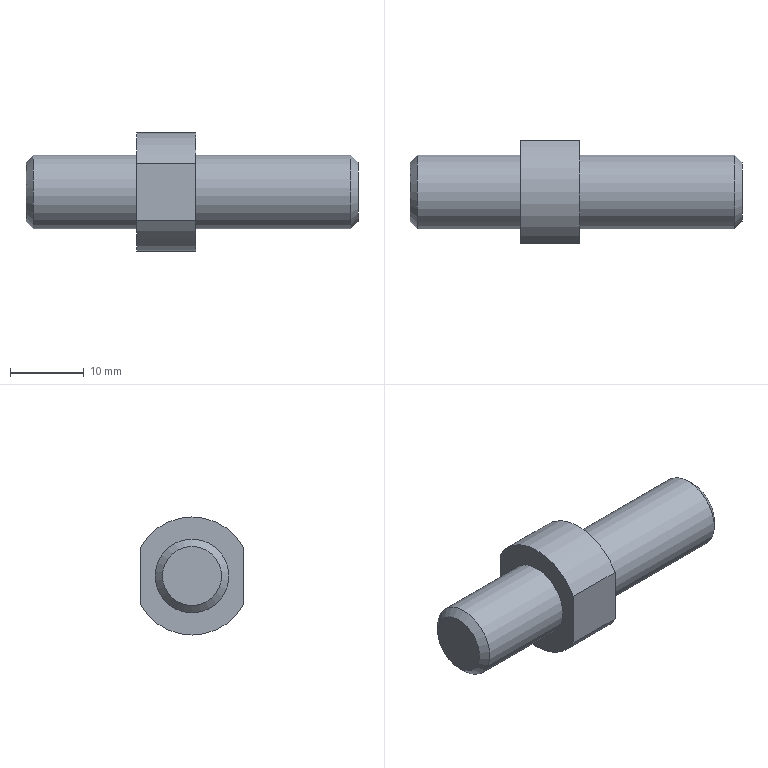Part | NX | 1 solid | 14 faces | box 45 x 14 x 16 mm | volume 4202 mm3 | plane 6 | cylinder 5 | cone 3 | commonest cylinder face diameters 10 x2 16 x2 4.2 x1
STEP:
#1=CARTESIAN_POINT('',(-19.,0.,5.));
#2=VERTEX_POINT('',#1);
#3=CARTESIAN_POINT('',(-19.,0.,0.));
#4=DIRECTION('',(-1.,0.,0.));
#5=DIRECTION('',(0.,0.,1.));
#6=AXIS2_PLACEMENT_3D('',#3,#4,#5);
#7=CIRCLE('',#6,5.);
#8=EDGE_CURVE('',#2,#2,#7,.T.);
#9=ORIENTED_EDGE('',*,*,#8,.F.);
#10=EDGE_LOOP('',(#9));
#11=FACE_BOUND('',#10,.T.);
#12=CARTESIAN_POINT('',(-19.,7.,-3.873));
#13=VERTEX_POINT('',#12);
#14=CARTESIAN_POINT('',(-19.,-7.,-3.873));
#15=VERTEX_POINT('',#14);
#16=CARTESIAN_POINT('',(-19.,0.,0.));
#17=DIRECTION('',(-1.,0.,0.));
#18=DIRECTION('',(0.,0.,1.));
#19=AXIS2_PLACEMENT_3D('',#16,#17,#18);
#20=CIRCLE('',#19,8.);
#21=EDGE_CURVE('',#13,#15,#20,.T.);
#22=ORIENTED_EDGE('',*,*,#21,.T.);
#23=CARTESIAN_POINT('',(-19.,-7.,3.873));
#24=VERTEX_POINT('',#23);
#25=CARTESIAN_POINT('',(-19.,-7.,0.));
#26=DIRECTION('',(0.,0.,1.));
#27=VECTOR('',#26,1000.);
#28=LINE('',#25,#27);
#29=EDGE_CURVE('',#15,#24,#28,.T.);
#30=ORIENTED_EDGE('',*,*,#29,.T.);
#31=CARTESIAN_POINT('',(-19.,7.,3.873));
#32=VERTEX_POINT('',#31);
#33=CARTESIAN_POINT('',(-19.,0.,0.));
#34=DIRECTION('',(-1.,0.,0.));
#35=DIRECTION('',(0.,0.,1.));
#36=AXIS2_PLACEMENT_3D('',#33,#34,#35);
#37=CIRCLE('',#36,8.);
#38=EDGE_CURVE('',#24,#32,#37,.T.);
#39=ORIENTED_EDGE('',*,*,#38,.T.);
#40=CARTESIAN_POINT('',(-19.,7.,0.));
#41=DIRECTION('',(0.,0.,-1.));
#42=VECTOR('',#41,1000.);
#43=LINE('',#40,#42);
#44=EDGE_CURVE('',#32,#13,#43,.T.);
#45=ORIENTED_EDGE('',*,*,#44,.T.);
#46=EDGE_LOOP('',(#22,#30,#39,#45));
#47=FACE_BOUND('',#46,.T.);
#48=CARTESIAN_POINT('',(-19.,0.,0.));
#49=DIRECTION('',(-1.,0.,0.));
#50=DIRECTION('',(0.,0.,1.));
#51=AXIS2_PLACEMENT_3D('',#48,#49,#50);
#52=PLANE('',#51);
#53=ADVANCED_FACE('',(#11,#47),#52,.T.);
#54=CARTESIAN_POINT('',(-11.,0.,5.));
#55=VERTEX_POINT('',#54);
#56=CARTESIAN_POINT('',(-11.,0.,0.));
#57=DIRECTION('',(-1.,0.,0.));
#58=DIRECTION('',(0.,0.,1.));
#59=AXIS2_PLACEMENT_3D('',#56,#57,#58);
#60=CIRCLE('',#59,5.);
#61=EDGE_CURVE('',#55,#55,#60,.T.);
#62=ORIENTED_EDGE('',*,*,#61,.T.);
#63=EDGE_LOOP('',(#62));
#64=FACE_BOUND('',#63,.T.);
#65=CARTESIAN_POINT('',(-11.,-7.,3.873));
#66=VERTEX_POINT('',#65);
#67=CARTESIAN_POINT('',(-11.,-7.,-3.873));
#68=VERTEX_POINT('',#67);
#69=CARTESIAN_POINT('',(-11.,-7.,12.5));
#70=DIRECTION('',(0.,0.,-1.));
#71=VECTOR('',#70,1000.);
#72=LINE('',#69,#71);
#73=EDGE_CURVE('',#66,#68,#72,.T.);
#74=ORIENTED_EDGE('',*,*,#73,.T.);
#75=CARTESIAN_POINT('',(-11.,7.,-3.873));
#76=VERTEX_POINT('',#75);
#77=CARTESIAN_POINT('',(-11.,0.,0.));
#78=DIRECTION('',(-1.,0.,0.));
#79=DIRECTION('',(0.,0.,1.));
#80=AXIS2_PLACEMENT_3D('',#77,#78,#79);
#81=CIRCLE('',#80,8.);
#82=EDGE_CURVE('',#76,#68,#81,.T.);
#83=ORIENTED_EDGE('',*,*,#82,.F.);
#84=CARTESIAN_POINT('',(-11.,7.,3.873));
#85=VERTEX_POINT('',#84);
#86=CARTESIAN_POINT('',(-11.,7.,12.5));
#87=DIRECTION('',(0.,0.,1.));
#88=VECTOR('',#87,1000.);
#89=LINE('',#86,#88);
#90=EDGE_CURVE('',#76,#85,#89,.T.);
#91=ORIENTED_EDGE('',*,*,#90,.T.);
#92=CARTESIAN_POINT('',(-11.,0.,0.));
#93=DIRECTION('',(-1.,0.,0.));
#94=DIRECTION('',(0.,0.,1.));
#95=AXIS2_PLACEMENT_3D('',#92,#93,#94);
#96=CIRCLE('',#95,8.);
#97=EDGE_CURVE('',#66,#85,#96,.T.);
#98=ORIENTED_EDGE('',*,*,#97,.F.);
#99=EDGE_LOOP('',(#74,#83,#91,#98));
#100=FACE_BOUND('',#99,.T.);
#101=CARTESIAN_POINT('',(-11.,0.,0.));
#102=DIRECTION('',(-1.,0.,0.));
#103=DIRECTION('',(0.,0.,1.));
#104=AXIS2_PLACEMENT_3D('',#101,#102,#103);
#105=PLANE('',#104);
#106=ADVANCED_FACE('',(#64,#100),#105,.F.);
#107=CARTESIAN_POINT('',(-19.,-7.,-3.873));
#108=DIRECTION('',(1.,0.,0.));
#109=VECTOR('',#108,1000.);
#110=LINE('',#107,#109);
#111=EDGE_CURVE('',#15,#68,#110,.T.);
#112=ORIENTED_EDGE('',*,*,#111,.F.);
#113=ORIENTED_EDGE('',*,*,#21,.F.);
#114=CARTESIAN_POINT('',(-19.,7.,-3.873));
#115=DIRECTION('',(1.,0.,0.));
#116=VECTOR('',#115,1000.);
#117=LINE('',#114,#116);
#118=EDGE_CURVE('',#76,#13,#117,.F.);
#119=ORIENTED_EDGE('',*,*,#118,.F.);
#120=ORIENTED_EDGE('',*,*,#82,.T.);
#121=EDGE_LOOP('',(#112,#113,#119,#120));
#122=FACE_BOUND('',#121,.T.);
#123=CARTESIAN_POINT('',(-19.,0.,0.));
#124=DIRECTION('',(1.,0.,0.));
#125=DIRECTION('',(0.,0.,-1.));
#126=AXIS2_PLACEMENT_3D('',#123,#124,#125);
#127=CYLINDRICAL_SURFACE('',#126,8.);
#128=ADVANCED_FACE('',(#122),#127,.T.);
#129=CARTESIAN_POINT('',(-19.,-7.,3.873));
#130=DIRECTION('',(1.,0.,0.));
#131=VECTOR('',#130,1000.);
#132=LINE('',#129,#131);
#133=EDGE_CURVE('',#66,#24,#132,.F.);
#134=ORIENTED_EDGE('',*,*,#133,.F.);
#135=ORIENTED_EDGE('',*,*,#97,.T.);
#136=CARTESIAN_POINT('',(-19.,7.,3.873));
#137=DIRECTION('',(1.,0.,0.));
#138=VECTOR('',#137,1000.);
#139=LINE('',#136,#138);
#140=EDGE_CURVE('',#32,#85,#139,.T.);
#141=ORIENTED_EDGE('',*,*,#140,.F.);
#142=ORIENTED_EDGE('',*,*,#38,.F.);
#143=EDGE_LOOP('',(#134,#135,#141,#142));
#144=FACE_BOUND('',#143,.T.);
#145=CARTESIAN_POINT('',(-19.,0.,0.));
#146=DIRECTION('',(1.,0.,0.));
#147=DIRECTION('',(0.,0.,-1.));
#148=AXIS2_PLACEMENT_3D('',#145,#146,#147);
#149=CYLINDRICAL_SURFACE('',#148,8.);
#150=ADVANCED_FACE('',(#144),#149,.T.);
#151=CARTESIAN_POINT('',(10.,0.,-5.));
#152=VERTEX_POINT('',#151);
#153=CARTESIAN_POINT('',(10.,0.,0.));
#154=DIRECTION('',(1.,0.,0.));
#155=DIRECTION('',(0.,0.,-1.));
#156=AXIS2_PLACEMENT_3D('',#153,#154,#155);
#157=CIRCLE('',#156,5.);
#158=EDGE_CURVE('',#152,#152,#157,.F.);
#159=ORIENTED_EDGE('',*,*,#158,.T.);
#160=EDGE_LOOP('',(#159));
#161=FACE_BOUND('',#160,.T.);
#162=ORIENTED_EDGE('',*,*,#61,.F.);
#163=EDGE_LOOP('',(#162));
#164=FACE_BOUND('',#163,.T.);
#165=CARTESIAN_POINT('',(11.,0.,0.));
#166=DIRECTION('',(-1.,0.,0.));
#167=DIRECTION('',(0.,0.,1.));
#168=AXIS2_PLACEMENT_3D('',#165,#166,#167);
#169=CYLINDRICAL_SURFACE('',#168,5.);
#170=ADVANCED_FACE('',(#161,#164),#169,.T.);
#171=CARTESIAN_POINT('',(11.,0.,-2.1));
#172=VERTEX_POINT('',#171);
#173=CARTESIAN_POINT('',(11.,0.,0.));
#174=DIRECTION('',(1.,0.,0.));
#175=DIRECTION('',(0.,0.,-1.));
#176=AXIS2_PLACEMENT_3D('',#173,#174,#175);
#177=CIRCLE('',#176,2.1);
#178=EDGE_CURVE('',#172,#172,#177,.T.);
#179=ORIENTED_EDGE('',*,*,#178,.F.);
#180=EDGE_LOOP('',(#179));
#181=FACE_BOUND('',#180,.T.);
#182=CARTESIAN_POINT('',(11.,0.,-4.));
#183=VERTEX_POINT('',#182);
#184=CARTESIAN_POINT('',(11.,0.,0.));
#185=DIRECTION('',(1.,0.,0.));
#186=DIRECTION('',(0.,0.,-1.));
#187=AXIS2_PLACEMENT_3D('',#184,#185,#186);
#188=CIRCLE('',#187,4.);
#189=EDGE_CURVE('',#183,#183,#188,.T.);
#190=ORIENTED_EDGE('',*,*,#189,.T.);
#191=EDGE_LOOP('',(#190));
#192=FACE_BOUND('',#191,.T.);
#193=CARTESIAN_POINT('',(11.,0.,0.));
#194=DIRECTION('',(1.,0.,0.));
#195=DIRECTION('',(0.,0.,-1.));
#196=AXIS2_PLACEMENT_3D('',#193,#194,#195);
#197=PLANE('',#196);
#198=ADVANCED_FACE('',(#181,#192),#197,.T.);
#199=CARTESIAN_POINT('',(-33.,0.,5.));
#200=VERTEX_POINT('',#199);
#201=CARTESIAN_POINT('',(-33.,0.,0.));
#202=DIRECTION('',(-1.,0.,0.));
#203=DIRECTION('',(0.,0.,1.));
#204=AXIS2_PLACEMENT_3D('',#201,#202,#203);
#205=CIRCLE('',#204,5.);
#206=EDGE_CURVE('',#200,#200,#205,.F.);
#207=ORIENTED_EDGE('',*,*,#206,.T.);
#208=EDGE_LOOP('',(#207));
#209=FACE_BOUND('',#208,.T.);
#210=ORIENTED_EDGE('',*,*,#8,.T.);
#211=EDGE_LOOP('',(#210));
#212=FACE_BOUND('',#211,.T.);
#213=CARTESIAN_POINT('',(-34.,0.,0.));
#214=DIRECTION('',(1.,0.,0.));
#215=DIRECTION('',(0.,0.,-1.));
#216=AXIS2_PLACEMENT_3D('',#213,#214,#215);
#217=CYLINDRICAL_SURFACE('',#216,5.);
#218=ADVANCED_FACE('',(#209,#212),#217,.T.);
#219=CARTESIAN_POINT('',(-34.,0.,4.));
#220=VERTEX_POINT('',#219);
#221=CARTESIAN_POINT('',(-34.,0.,0.));
#222=DIRECTION('',(-1.,0.,0.));
#223=DIRECTION('',(0.,0.,1.));
#224=AXIS2_PLACEMENT_3D('',#221,#222,#223);
#225=CIRCLE('',#224,4.);
#226=EDGE_CURVE('',#220,#220,#225,.T.);
#227=ORIENTED_EDGE('',*,*,#226,.T.);
#228=EDGE_LOOP('',(#227));
#229=FACE_BOUND('',#228,.T.);
#230=CARTESIAN_POINT('',(-34.,0.,0.));
#231=DIRECTION('',(-1.,0.,0.));
#232=DIRECTION('',(0.,0.,1.));
#233=AXIS2_PLACEMENT_3D('',#230,#231,#232);
#234=PLANE('',#233);
#235=ADVANCED_FACE('',(#229),#234,.T.);
#236=ORIENTED_EDGE('',*,*,#158,.F.);
#237=EDGE_LOOP('',(#236));
#238=FACE_BOUND('',#237,.T.);
#239=ORIENTED_EDGE('',*,*,#189,.F.);
#240=EDGE_LOOP('',(#239));
#241=FACE_BOUND('',#240,.T.);
#242=CARTESIAN_POINT('',(11.,0.,0.));
#243=DIRECTION('',(-1.,0.,0.));
#244=DIRECTION('',(0.,0.,1.));
#245=AXIS2_PLACEMENT_3D('',#242,#243,#244);
#246=CONICAL_SURFACE('',#245,4.,0.7854);
#247=ADVANCED_FACE('',(#238,#241),#246,.T.);
#248=ORIENTED_EDGE('',*,*,#206,.F.);
#249=EDGE_LOOP('',(#248));
#250=FACE_BOUND('',#249,.T.);
#251=ORIENTED_EDGE('',*,*,#226,.F.);
#252=EDGE_LOOP('',(#251));
#253=FACE_BOUND('',#252,.T.);
#254=CARTESIAN_POINT('',(-34.,0.,0.));
#255=DIRECTION('',(1.,0.,0.));
#256=DIRECTION('',(0.,0.,-1.));
#257=AXIS2_PLACEMENT_3D('',#254,#255,#256);
#258=CONICAL_SURFACE('',#257,4.,0.7854);
#259=ADVANCED_FACE('',(#250,#253),#258,.T.);
#260=ORIENTED_EDGE('',*,*,#140,.T.);
#261=ORIENTED_EDGE('',*,*,#90,.F.);
#262=ORIENTED_EDGE('',*,*,#118,.T.);
#263=ORIENTED_EDGE('',*,*,#44,.F.);
#264=EDGE_LOOP('',(#260,#261,#262,#263));
#265=FACE_BOUND('',#264,.T.);
#266=CARTESIAN_POINT('',(-34.,7.,12.5));
#267=DIRECTION('',(0.,1.,0.));
#268=DIRECTION('',(0.,0.,1.));
#269=AXIS2_PLACEMENT_3D('',#266,#267,#268);
#270=PLANE('',#269);
#271=ADVANCED_FACE('',(#265),#270,.T.);
#272=ORIENTED_EDGE('',*,*,#111,.T.);
#273=ORIENTED_EDGE('',*,*,#73,.F.);
#274=ORIENTED_EDGE('',*,*,#133,.T.);
#275=ORIENTED_EDGE('',*,*,#29,.F.);
#276=EDGE_LOOP('',(#272,#273,#274,#275));
#277=FACE_BOUND('',#276,.T.);
#278=CARTESIAN_POINT('',(-34.,-7.,12.5));
#279=DIRECTION('',(0.,-1.,0.));
#280=DIRECTION('',(0.,0.,-1.));
#281=AXIS2_PLACEMENT_3D('',#278,#279,#280);
#282=PLANE('',#281);
#283=ADVANCED_FACE('',(#277),#282,.T.);
#284=CARTESIAN_POINT('',(-4.262,0.,0.));
#285=VERTEX_POINT('',#284);
#286=VERTEX_LOOP('',#285);
#287=FACE_BOUND('',#286,.T.);
#288=CARTESIAN_POINT('',(-3.,0.,-2.1));
#289=VERTEX_POINT('',#288);
#290=CARTESIAN_POINT('',(-3.,0.,0.));
#291=DIRECTION('',(1.,0.,0.));
#292=DIRECTION('',(0.,0.,-1.));
#293=AXIS2_PLACEMENT_3D('',#290,#291,#292);
#294=CIRCLE('',#293,2.1);
#295=EDGE_CURVE('',#289,#289,#294,.T.);
#296=ORIENTED_EDGE('',*,*,#295,.T.);
#297=EDGE_LOOP('',(#296));
#298=FACE_BOUND('',#297,.T.);
#299=CARTESIAN_POINT('',(-3.,0.,0.));
#300=DIRECTION('',(1.,0.,0.));
#301=DIRECTION('',(0.,0.,-1.));
#302=AXIS2_PLACEMENT_3D('',#299,#300,#301);
#303=CONICAL_SURFACE('',#302,2.1,1.03);
#304=ADVANCED_FACE('',(#287,#298),#303,.F.);
#305=ORIENTED_EDGE('',*,*,#295,.F.);
#306=EDGE_LOOP('',(#305));
#307=FACE_BOUND('',#306,.T.);
#308=ORIENTED_EDGE('',*,*,#178,.T.);
#309=EDGE_LOOP('',(#308));
#310=FACE_BOUND('',#309,.T.);
#311=CARTESIAN_POINT('',(11.,0.,0.));
#312=DIRECTION('',(1.,0.,0.));
#313=DIRECTION('',(0.,0.,-1.));
#314=AXIS2_PLACEMENT_3D('',#311,#312,#313);
#315=CYLINDRICAL_SURFACE('',#314,2.1);
#316=ADVANCED_FACE('',(#307,#310),#315,.F.);
#317=CLOSED_SHELL('',(#53,#106,#128,#150,#170,#198,#218,#235,#247,#259,#271,#283,#304,#316));
#318=MANIFOLD_SOLID_BREP('',#317);
#319=(LENGTH_UNIT()NAMED_UNIT(*)SI_UNIT(.MILLI.,.METRE.));
#320=UNCERTAINTY_MEASURE_WITH_UNIT(LENGTH_MEASURE(0.00001),#319,'','');
#321=(NAMED_UNIT(*)PLANE_ANGLE_UNIT()SI_UNIT($,.RADIAN.));
#322=(NAMED_UNIT(*)SI_UNIT($,.STERADIAN.)SOLID_ANGLE_UNIT());
#323=(GEOMETRIC_REPRESENTATION_CONTEXT(3)GLOBAL_UNCERTAINTY_ASSIGNED_CONTEXT((#320))GLOBAL_UNIT_ASSIGNED_CONTEXT((#319,#321,#322))REPRESENTATION_CONTEXT('',''));
#324=ADVANCED_BREP_SHAPE_REPRESENTATION('',(#318),#323);